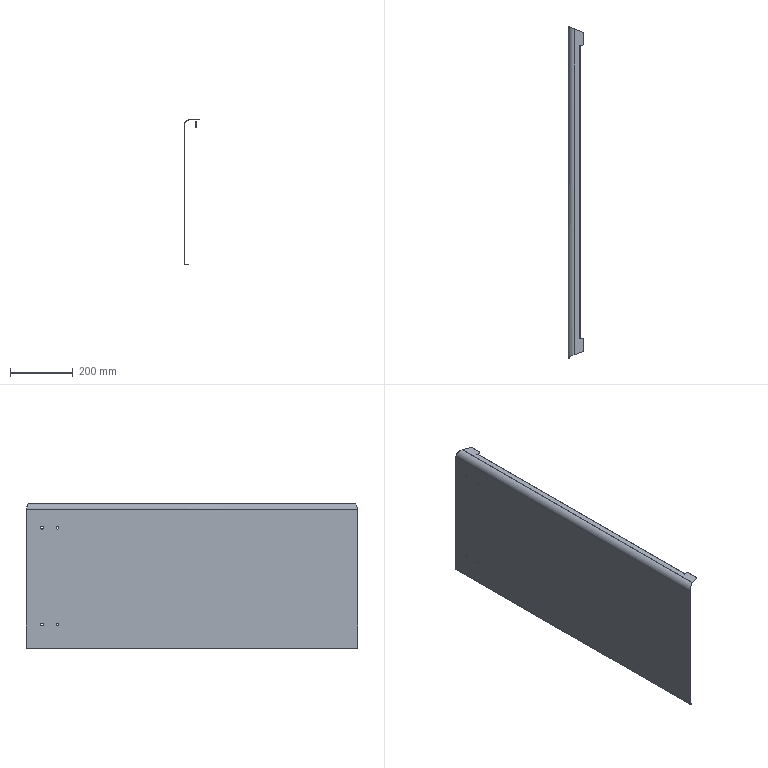Part | SolidWorks | features EdgeFlange 3, FlatPattern 1, HoleWzd 1, SMBaseFlange 1, SheetMetal 1 | 1 solid | 54 faces | box 50 x 1055 x 460.8 mm | volume 442365 mm3 | plane 34 | cylinder 18 | spline 2 | commonest cylinder face diameters 9 x8 10 x4 1 x2 2.6 x2 38.4 x1 40 x1